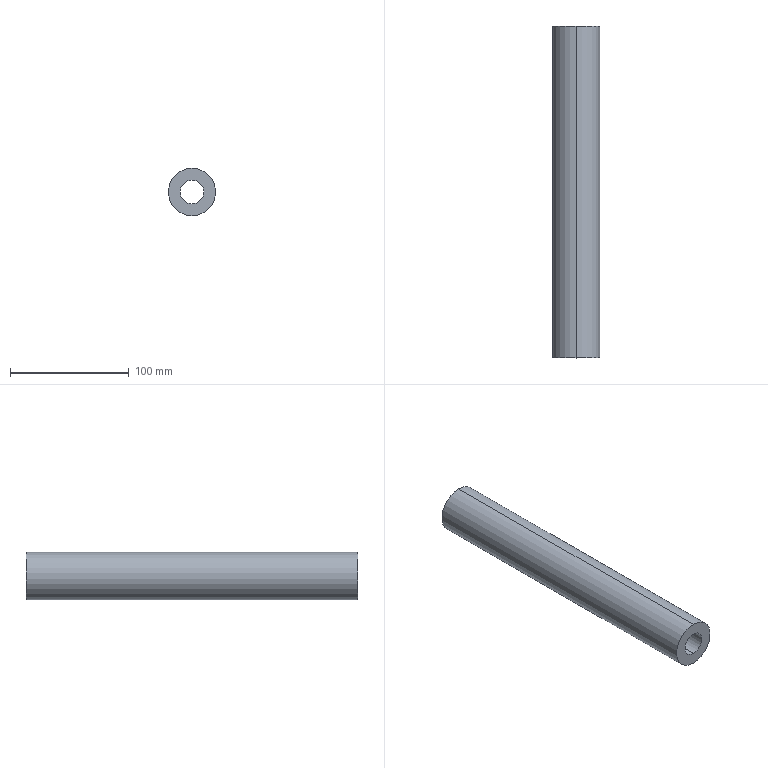Part | SolidWorks | features Extrusion 1 | 1 solid | 6 faces | box 40 x 280 x 40 mm | volume 263894 mm3 | cylinder 4 | plane 2 | commonest cylinder face diameters 20 x2 40 x2
STEP:
#1=CARTESIAN_POINT('',(0.,140.,-10.));
#2=VERTEX_POINT('',#1);
#3=CARTESIAN_POINT('',(0.,140.,10.));
#4=VERTEX_POINT('',#3);
#5=CARTESIAN_POINT('',(0.,140.,0.));
#6=DIRECTION('',(0.,1.,0.));
#7=DIRECTION('',(0.,0.,1.));
#8=AXIS2_PLACEMENT_3D('',#5,#6,#7);
#9=CIRCLE('',#8,10.);
#10=EDGE_CURVE('',#2,#4,#9,.T.);
#11=ORIENTED_EDGE('',*,*,#10,.T.);
#12=CARTESIAN_POINT('',(0.,-140.,10.));
#13=VERTEX_POINT('',#12);
#14=CARTESIAN_POINT('',(0.,140.,10.));
#15=DIRECTION('',(0.,-1.,0.));
#16=VECTOR('',#15,1000.);
#17=LINE('',#14,#16);
#18=EDGE_CURVE('',#4,#13,#17,.T.);
#19=ORIENTED_EDGE('',*,*,#18,.T.);
#20=CARTESIAN_POINT('',(0.,-140.,-10.));
#21=VERTEX_POINT('',#20);
#22=CARTESIAN_POINT('',(0.,-140.,0.));
#23=DIRECTION('',(0.,1.,0.));
#24=DIRECTION('',(0.,0.,1.));
#25=AXIS2_PLACEMENT_3D('',#22,#23,#24);
#26=CIRCLE('',#25,10.);
#27=EDGE_CURVE('',#21,#13,#26,.T.);
#28=ORIENTED_EDGE('',*,*,#27,.F.);
#29=CARTESIAN_POINT('',(0.,140.,-10.));
#30=DIRECTION('',(0.,-1.,0.));
#31=VECTOR('',#30,1000.);
#32=LINE('',#29,#31);
#33=EDGE_CURVE('',#2,#21,#32,.T.);
#34=ORIENTED_EDGE('',*,*,#33,.F.);
#35=EDGE_LOOP('',(#11,#19,#28,#34));
#36=FACE_OUTER_BOUND('',#35,.T.);
#37=CARTESIAN_POINT('',(0.,140.,0.));
#38=DIRECTION('',(0.,-1.,0.));
#39=DIRECTION('',(0.,0.,-1.));
#40=AXIS2_PLACEMENT_3D('',#37,#38,#39);
#41=CYLINDRICAL_SURFACE('',#40,10.);
#42=ADVANCED_FACE('',(#36),#41,.F.);
#43=CARTESIAN_POINT('',(0.,140.,20.));
#44=VERTEX_POINT('',#43);
#45=CARTESIAN_POINT('',(0.,140.,-20.));
#46=VERTEX_POINT('',#45);
#47=CARTESIAN_POINT('',(0.,140.,0.));
#48=DIRECTION('',(0.,1.,0.));
#49=DIRECTION('',(0.,0.,1.));
#50=AXIS2_PLACEMENT_3D('',#47,#48,#49);
#51=CIRCLE('',#50,20.);
#52=EDGE_CURVE('',#44,#46,#51,.T.);
#53=ORIENTED_EDGE('',*,*,#52,.F.);
#54=CARTESIAN_POINT('',(0.,-140.,20.));
#55=VERTEX_POINT('',#54);
#56=CARTESIAN_POINT('',(0.,140.,20.));
#57=DIRECTION('',(0.,-1.,0.));
#58=VECTOR('',#57,1000.);
#59=LINE('',#56,#58);
#60=EDGE_CURVE('',#44,#55,#59,.T.);
#61=ORIENTED_EDGE('',*,*,#60,.T.);
#62=CARTESIAN_POINT('',(0.,-140.,-20.));
#63=VERTEX_POINT('',#62);
#64=CARTESIAN_POINT('',(0.,-140.,0.));
#65=DIRECTION('',(0.,1.,0.));
#66=DIRECTION('',(0.,0.,1.));
#67=AXIS2_PLACEMENT_3D('',#64,#65,#66);
#68=CIRCLE('',#67,20.);
#69=EDGE_CURVE('',#55,#63,#68,.T.);
#70=ORIENTED_EDGE('',*,*,#69,.T.);
#71=CARTESIAN_POINT('',(0.,140.,-20.));
#72=DIRECTION('',(0.,-1.,0.));
#73=VECTOR('',#72,1000.);
#74=LINE('',#71,#73);
#75=EDGE_CURVE('',#46,#63,#74,.T.);
#76=ORIENTED_EDGE('',*,*,#75,.F.);
#77=EDGE_LOOP('',(#53,#61,#70,#76));
#78=FACE_OUTER_BOUND('',#77,.T.);
#79=CARTESIAN_POINT('',(0.,140.,0.));
#80=DIRECTION('',(0.,-1.,0.));
#81=DIRECTION('',(0.,0.,-1.));
#82=AXIS2_PLACEMENT_3D('',#79,#80,#81);
#83=CYLINDRICAL_SURFACE('',#82,20.);
#84=ADVANCED_FACE('',(#78),#83,.T.);
#85=CARTESIAN_POINT('',(0.,140.,0.));
#86=DIRECTION('',(0.,1.,0.));
#87=DIRECTION('',(0.,0.,1.));
#88=AXIS2_PLACEMENT_3D('',#85,#86,#87);
#89=CIRCLE('',#88,20.);
#90=EDGE_CURVE('',#46,#44,#89,.T.);
#91=ORIENTED_EDGE('',*,*,#90,.T.);
#92=ORIENTED_EDGE('',*,*,#52,.T.);
#93=EDGE_LOOP('',(#91,#92));
#94=FACE_OUTER_BOUND('',#93,.T.);
#95=ORIENTED_EDGE('',*,*,#10,.F.);
#96=CARTESIAN_POINT('',(0.,140.,0.));
#97=DIRECTION('',(0.,1.,0.));
#98=DIRECTION('',(0.,0.,1.));
#99=AXIS2_PLACEMENT_3D('',#96,#97,#98);
#100=CIRCLE('',#99,10.);
#101=EDGE_CURVE('',#4,#2,#100,.T.);
#102=ORIENTED_EDGE('',*,*,#101,.F.);
#103=EDGE_LOOP('',(#95,#102));
#104=FACE_BOUND('',#103,.T.);
#105=CARTESIAN_POINT('',(0.,140.,0.));
#106=DIRECTION('',(0.,1.,0.));
#107=DIRECTION('',(0.,0.,1.));
#108=AXIS2_PLACEMENT_3D('',#105,#106,#107);
#109=PLANE('',#108);
#110=ADVANCED_FACE('',(#94,#104),#109,.T.);
#111=CARTESIAN_POINT('',(0.,-140.,0.));
#112=DIRECTION('',(0.,1.,0.));
#113=DIRECTION('',(0.,0.,1.));
#114=AXIS2_PLACEMENT_3D('',#111,#112,#113);
#115=CIRCLE('',#114,20.);
#116=EDGE_CURVE('',#63,#55,#115,.T.);
#117=ORIENTED_EDGE('',*,*,#116,.F.);
#118=ORIENTED_EDGE('',*,*,#69,.F.);
#119=EDGE_LOOP('',(#117,#118));
#120=FACE_OUTER_BOUND('',#119,.T.);
#121=ORIENTED_EDGE('',*,*,#27,.T.);
#122=CARTESIAN_POINT('',(0.,-140.,0.));
#123=DIRECTION('',(0.,1.,0.));
#124=DIRECTION('',(0.,0.,1.));
#125=AXIS2_PLACEMENT_3D('',#122,#123,#124);
#126=CIRCLE('',#125,10.);
#127=EDGE_CURVE('',#13,#21,#126,.T.);
#128=ORIENTED_EDGE('',*,*,#127,.T.);
#129=EDGE_LOOP('',(#121,#128));
#130=FACE_BOUND('',#129,.T.);
#131=CARTESIAN_POINT('',(0.,-140.,0.));
#132=DIRECTION('',(0.,1.,0.));
#133=DIRECTION('',(0.,0.,1.));
#134=AXIS2_PLACEMENT_3D('',#131,#132,#133);
#135=PLANE('',#134);
#136=ADVANCED_FACE('',(#120,#130),#135,.F.);
#137=ORIENTED_EDGE('',*,*,#60,.F.);
#138=ORIENTED_EDGE('',*,*,#90,.F.);
#139=ORIENTED_EDGE('',*,*,#75,.T.);
#140=ORIENTED_EDGE('',*,*,#116,.T.);
#141=EDGE_LOOP('',(#137,#138,#139,#140));
#142=FACE_OUTER_BOUND('',#141,.T.);
#143=CARTESIAN_POINT('',(0.,140.,0.));
#144=DIRECTION('',(0.,-1.,0.));
#145=DIRECTION('',(0.,0.,-1.));
#146=AXIS2_PLACEMENT_3D('',#143,#144,#145);
#147=CYLINDRICAL_SURFACE('',#146,20.);
#148=ADVANCED_FACE('',(#142),#147,.T.);
#149=ORIENTED_EDGE('',*,*,#18,.F.);
#150=ORIENTED_EDGE('',*,*,#101,.T.);
#151=ORIENTED_EDGE('',*,*,#33,.T.);
#152=ORIENTED_EDGE('',*,*,#127,.F.);
#153=EDGE_LOOP('',(#149,#150,#151,#152));
#154=FACE_OUTER_BOUND('',#153,.T.);
#155=CARTESIAN_POINT('',(0.,140.,0.));
#156=DIRECTION('',(0.,-1.,0.));
#157=DIRECTION('',(0.,0.,-1.));
#158=AXIS2_PLACEMENT_3D('',#155,#156,#157);
#159=CYLINDRICAL_SURFACE('',#158,10.);
#160=ADVANCED_FACE('',(#154),#159,.F.);
#161=CLOSED_SHELL('',(#42,#84,#110,#136,#148,#160));
#162=MANIFOLD_SOLID_BREP('',#161);
#163=CARTESIAN_POINT('',(0.,0.,0.));
#164=DIRECTION('',(0.,0.,1.));
#165=DIRECTION('',(1.,0.,0.));
#166=AXIS2_PLACEMENT_3D('',#163,#164,#165);
#167=(LENGTH_UNIT()NAMED_UNIT(*)SI_UNIT(.MILLI.,.METRE.));
#168=UNCERTAINTY_MEASURE_WITH_UNIT(LENGTH_MEASURE(0.00001),#167,'','');
#169=(NAMED_UNIT(*)PLANE_ANGLE_UNIT()SI_UNIT($,.RADIAN.));
#170=(NAMED_UNIT(*)SI_UNIT($,.STERADIAN.)SOLID_ANGLE_UNIT());
#171=(GEOMETRIC_REPRESENTATION_CONTEXT(3)GLOBAL_UNCERTAINTY_ASSIGNED_CONTEXT((#168))GLOBAL_UNIT_ASSIGNED_CONTEXT((#167,#169,#170))REPRESENTATION_CONTEXT('',''));
#172=ADVANCED_BREP_SHAPE_REPRESENTATION('',(#162,#166),#171);